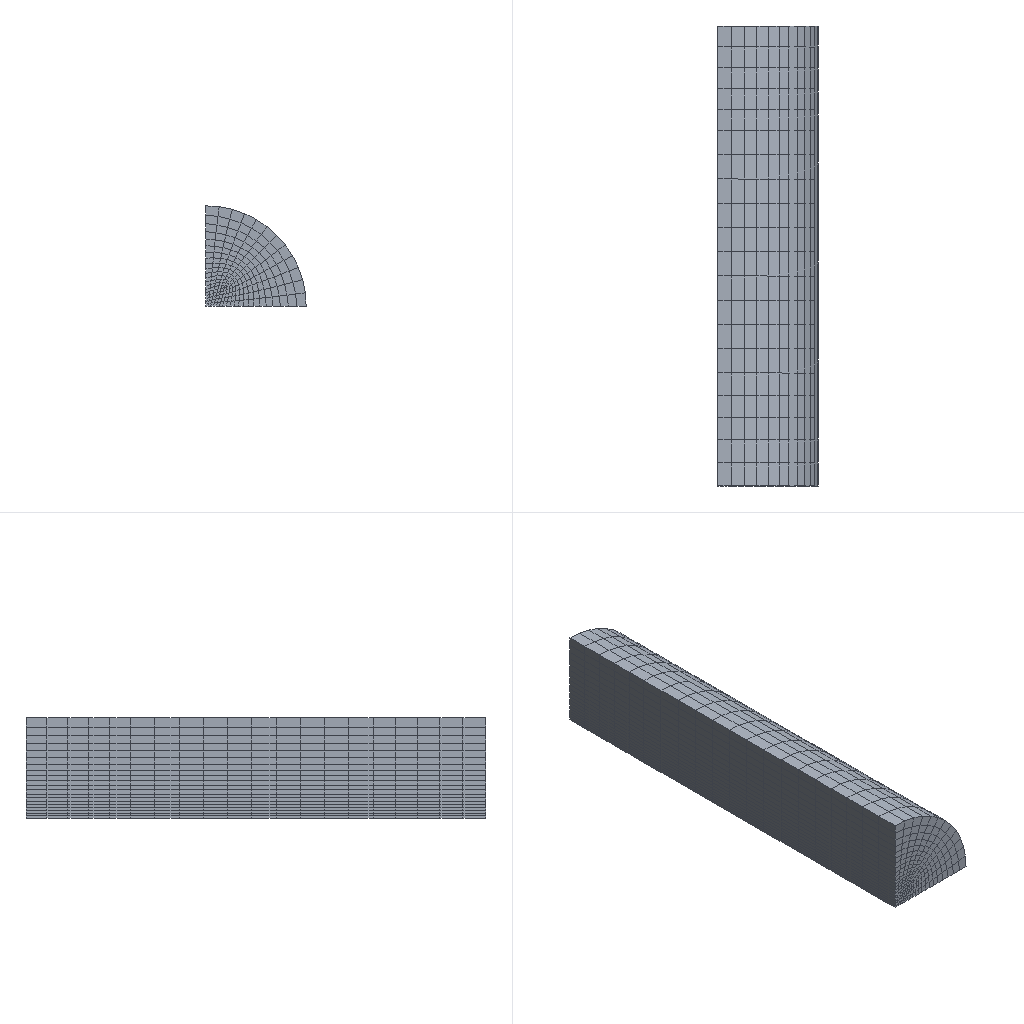Simulation study | abaqus
Set-up summary:
category,name,step,type,value,unit,region
solver,abaqus
solver,version,,,Abaqus/Explicit 2020
units,not stated in the deck,,not stated
analysis,deck,,transient,transient
load_step,Step-1,Step-1,transient
load_step,Step-2,Step-2,transient
load_step,requested,,,2
mesh,nodes,,,5486
mesh,elements,,,4714
element_type,R3D3,,rigid,4
element_type,R3D4,,rigid,630
element_type,EC3D8R,,solid,4080
load,load commands in deck,,count,2
bc,support commands in deck,,count,14
material,SOIL,,in results
material,SOIL-2,,in results
material,SOIL-3,,in results
material,SOIL-4,,in results
check,setup vs results,,match,"per instance, exact: element labels, types and connectivity; labels of the nodes the elements use; coordinates of those nodes at SINGLE_PRECISION in 2 of 2 instance(s)"
Abaqus input file, long lists of numbers shortened:
*Heading
** Job name: Job-1 Model name: Model-1
** Generated by: Abaqus/CAE 2020
*Preprint, echo=NO, model=NO, history=NO, contact=NO
**
** PARTS
**
*Part, name=PILE
*Node
      1,  0.2,  0.1155,           0.
      2,  0.2,   45.115,           0.
** (632 more lines like these left out)
*Element, type=R3D4
  1,   1,  15,  72,  16
  2,  15,  14,  73,  72
** (628 more lines like these left out)
*Element, type=R3D3
586, 603, 612, 611
587, 614, 601, 615
** (2 more lines like these left out)
*Node
    635,           0.,   45.115, 1.22464677e-17
*Nset, nset=PILE-RefPt_, internal
635,
*Elset, elset=PILE, generate
   1,  634,    1
*End Part
**
*Part, name=soil
*Node
      1,           0.,         13.5,           0.
      2,           0.,         13.5,          12.
** (4849 more lines like these left out)
*Element, type=EC3D8R
   1,   62,   63,  382,  368,  729,  730, 2191, 2177
   2,   63,   64,  383,  382,  730,  731, 2192, 2191
** (4078 more lines like these left out)
*Nset, nset=Set-1, generate
    1,  4851,     1
*Elset, elset=Set-1, generate
    1,  4080,     1
** Section: Section-1
*Eulerian Section, elset=Set-1
soil, soil-1
soil-2, soil-2-1
soil-3, soil-3-1
soil-4, soil-4-1
*Surface, type=EULERIAN MATERIAL, name=soil-1
soil-1
*Surface, type=EULERIAN MATERIAL, name=soil-2-1
soil-2-1
*Surface, type=EULERIAN MATERIAL, name=soil-3-1
soil-3-1
*Surface, type=EULERIAN MATERIAL, name=soil-4-1
soil-4-1
*End Part
**
**
** ASSEMBLY
**
*Assembly, name=Assembly
**
*Instance, name=PILE-1, part=PILE
          0.,          50.,           0.
*End Instance
**
*Instance, name=soil-1, part=soil
*End Instance
**
*Nset, nset=Set-1, instance=soil-1
    1,    2,    3,    4,    5,    6,    7,    8,    9,   13,   14,   15,   16,   17,   18,   19
   20,   21,   22,   23,   24,   25,   26,   27,   28,   29,   30,   31,   32,   33,   34,   35
** (273 more lines like these left out)
*Elset, elset=Set-1, instance=soil-1
    1,    2,    3,    4,    5,    6,    7,    8,    9,   10,   11,   12,   13,   14,   15,   16
   17,   18,   19,   20,   21,   22,   23,   24,   25,   26,   27,   28,   29,   30,   31,   32
** (228 more lines like these left out)
*Nset, nset=Set-2, instance=soil-1
    1,    3,    4,    6,    7,    9,   10,   12,   13,   15,   17,   18,   49,   50,   51,   52
   53,   54,   55,   56,   57,   58,   59,   60,   61,   62,   63,   64,   65,   66,   67,   68
** (26 more lines like these left out)
*Elset, elset=Set-2, instance=soil-1
    1,    2,    3,    4,    5,    6,  126,  132,  138,  144,  150,  156,  162,  168,  174,  180
  186,  192,  198,  204,  205,  206,  207,  208,  209,  210,  330,  336,  342,  348,  354,  360
** (23 more lines like these left out)
*Nset, nset=Set-3, instance=soil-1
    1,    2,    4,    5,    7,    8,   10,   11,   13,   14,   16,   17,   19,   20,   21,   22
   23,   24,   25,   26,   27,   28,   29,   30,   31,   32,   33,   34,   35,   36,   37,   68
** (26 more lines like these left out)
*Elset, elset=Set-3, instance=soil-1
    6,   12,   18,   24,   30,   36,   37,   38,   39,   40,   41,   42,   43,   44,   45,   46
   47,   48,   49,   50,  210,  216,  222,  228,  234,  240,  241,  242,  243,  244,  245,  246
** (23 more lines like these left out)
*Nset, nset=Set-4, instance=soil-1
   16,   17,   18,  309,  310,  311,  312,  313,  314,  315,  316,  317,  318,  319,  320,  321
  322,  323,  324,  325,  326,  327,  328,  329,  330,  331,  332,  333,  334,  335,  336,  337
** (13 more lines like these left out)
*Elset, elset=Set-4, instance=soil-1, generate
 3877,  4080,     1
*Nset, nset=Set-5, instance=soil-1, generate
    1,  4851,     1
*Elset, elset=Set-5, instance=soil-1, generate
    1,  4080,     1
*Nset, nset=Set-6, instance=soil-1
   13,   14,   15,   16,   17,   18,  257,  258,  259,  260,  261,  262,  263,  264,  265,  266
  267,  268,  269,  270,  271,  272,  273,  274,  275,  276,  277,  278,  279,  280,  281,  282
** (42 more lines like these left out)
*Elset, elset=Set-6, instance=soil-1, generate
 3673,  4080,     1
*Nset, nset=Set-7, instance=soil-1
    1,    2,    3,   13,   14,   15,   19,   20,   21,   22,   23,   24,   25,   26,   27,   28
   29,   30,   31,   32,   33,   34,   35,   36,   37,   38,   39,   40,   41,   42,   43,   44
** (56 more lines like these left out)
*Elset, elset=Set-7, instance=soil-1, generate
 3061,  3672,     1
*Nset, nset=Set-8, instance=soil-1
    1,    2,    3,    4,    5,    6,   19,   20,   21,   22,   23,   24,   25,   26,   27,   28
   29,   30,   31,   32,   33,   34,   35,   36,   37,   38,   39,   40,   41,   42,   43,   44
** (157 more lines like these left out)
*Elset, elset=Set-8, instance=soil-1, generate
    1,  2040,     1
*Nset, nset=Set-9, instance=soil-1
    4,    5,    6,    7,    8,    9,   95,   96,   97,   98,   99,  100,  101,  102,  103,  104
  105,  106,  107,  108,  109,  110,  111,  112,  113,  114,  115,  116,  117,  118,  119,  120
** (56 more lines like these left out)
*Elset, elset=Set-9, instance=soil-1, generate
 2041,  2652,     1
*Nset, nset=Set-10, instance=PILE-1
 635,
*Rigid Body, ref node=PILE-1.PILE-RefPt_, elset=PILE-1.PILE
*End Assembly
*Amplitude, name=Amp-1
             0.,              0.,             0.1,              1.
**
** MATERIALS
**
*Material, name=soil
*Density
1712.,
*Elastic
 1.5e+07, 0.49
*Mohr Coulomb
 15.8, 0.1
*Mohr Coulomb Hardening
4200.,0.
*Material, name=soil-2
*Density
1810.,
*Elastic
 4.7e+06, 0.49
*Mohr Coulomb
25., 0.1
*Mohr Coulomb Hardening
6130.,0.
*Material, name=soil-3
*Density
1920.,
*Elastic
 2e+07, 0.49
*Mohr Coulomb
20., 0.1
*Mohr Coulomb Hardening
10000.,0.
*Material, name=soil-4
*Density
2000.,
*Elastic
 3e+08, 0.3
*Mohr Coulomb
35., 0.1
*Mohr Coulomb Hardening
8000.,0.
**
** INTERACTION PROPERTIES
**
*Surface Interaction, name=IntProp-1
*Friction
 0.2,
*Surface Behavior, pressure-overclosure=HARD
**
** BOUNDARY CONDITIONS
**
** Name: BC-1 Type: 速度/角速度
*Boundary, type=VELOCITY
Set-2, 3, 3
Set-2, 4, 4
Set-2, 5, 5
** Name: BC-2 Type: 速度/角速度
*Boundary, type=VELOCITY
Set-3, 1, 1
Set-3, 5, 5
Set-3, 6, 6
** Name: BC-3 Type: 速度/角速度
*Boundary, type=VELOCITY
Set-4, 2, 2
**
** PREDEFINED FIELDS
**
** Name: Predefined Field-1   Type: Material assignment
*Initial Conditions, type=VOLUME FRACTION
Set-9, soil-1.soil-1, 1.
Set-8, soil-1.soil-2-1, 1.
Set-7, soil-1.soil-3-1, 1.
Set-6, soil-1.soil-4-1, 1.
**
** INTERACTIONS
**
** Interaction: Int-1
*Contact, op=NEW
*Contact Inclusions, ALL EXTERIOR
*Contact Property Assignment
 ,  , IntProp-1
** ----------------------------------------------------------------
**
** STEP: Step-1
**
*Step, name=Step-1, nlgeom=YES
*Dynamic, Explicit
, 0.1
*Bulk Viscosity
0.06, 1.2
**
** BOUNDARY CONDITIONS
**
** Name: [REDACTED] : Displacement/rotation angle
*Boundary, amplitude=Amp-1
Set-10, 1, 1
Set-10, 2, 2
Set-10, 3, 3
Set-10, 4, 4
Set-10, 5, 5
Set-10, 6, 6
**
** LOADS
**
** Name: Load-1   Type: Gravity
*Dload
Set-5, GRAV, 9.8, 0., -1., 0.
**
** OUTPUT REQUESTS
**
*Restart, write, number interval=1, time marks=NO
**
** FIELD OUTPUT: F-Output-1
**
*Output, field, number interval=100
*Node Output
A, CF, RF, RM, RT, U, V
*Element Output, directions=YES
DENSITYVAVG, EVF, EVOL, FV, LE, MISES, MISESMAX, MISESONLY, PE, PEEQ, PEEQVAVG, PEVAVG, PRESSONLY, S, SF, SSAVG
SVAVG, SVOL, TSHR
*Contact Output
CDISP, CFORCE, CSTRESS, FSLIP
**
** HISTORY OUTPUT: H-Output-1
**
*Output, history, variable=PRESELECT, frequency=1
*End Step
** ----------------------------------------------------------------
**
** STEP: Step-2
**
*Step, name=Step-2, nlgeom=YES
*Dynamic, Explicit
, 0.1
*Bulk Viscosity
0.06, 1.2
** Mass Scaling: Semi-Automatic
**               Whole Model
*Fixed Mass Scaling, factor=500.
**
** BOUNDARY CONDITIONS
**
** Name: [REDACTED] : Displacement/rotation angle
*Boundary, amplitude=Amp-1
Set-10, 2, 2, -47.
**
** OUTPUT REQUESTS
**
*Restart, write, number interval=1, time marks=NO
**
** FIELD OUTPUT: F-Output-1
**
*Output, field, number interval=100
*Node Output
A, CF, RF, RM, RT, U, V
*Element Output, directions=YES
DENSITYVAVG, EVF, EVOL, FV, LE, MISES, MISESMAX, MISESONLY, PE, PEEQ, PEEQVAVG, PEVAVG, PRESSONLY, S, SF, SSAVG
SVAVG, SVOL, TSHR
*Contact Output
CDISP, CFORCE, CSTRESS, FSLIP
**
** HISTORY OUTPUT: H-Output-1
**
*Output, history, variable=PRESELECT, frequency=1
*End Step
Results summary:
result,step,Step-1,completed,increments=284 time=0.1/0.1
result,step,Step-2,completed,increments=336 time=0.1/0.1
result,analysis,,,transient
result,last_loadstep,,,2
result,primary field,,,U
result,reaction total,,FX,300748991.129,model units
result,reaction total,,FY,-87698544.672,model units
result,reaction total,,FZ,286477945.116,model units